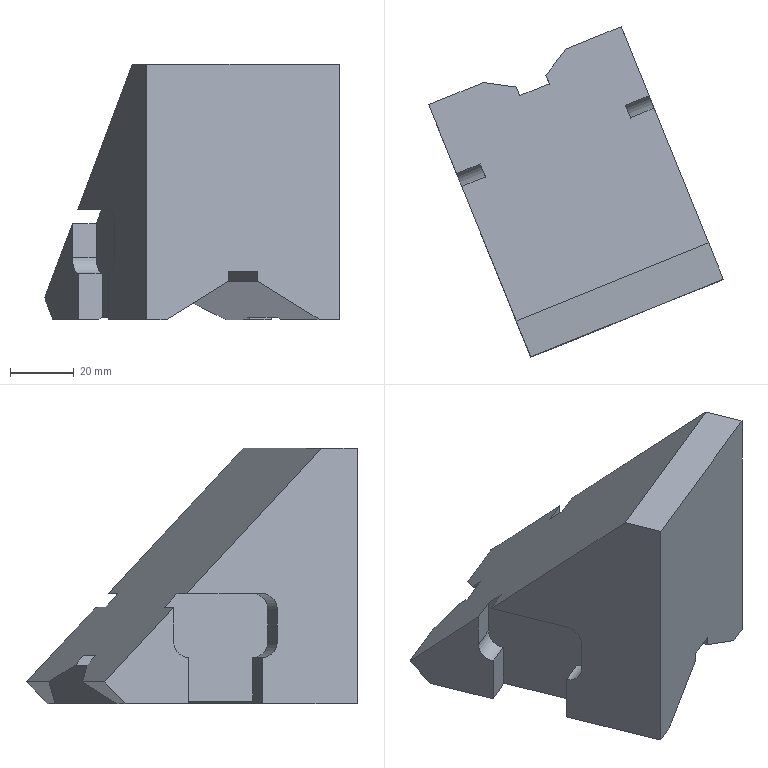Part | NX | features solid 2 | 1 solid | 36 faces | box 92.211 x 103.489 x 80 mm | volume 218804 mm3 | plane 30 | cylinder 6 | commonest cylinder face diameters 10 x6
STEP:
#1=CARTESIAN_POINT('',(-698.833,418.768,71.5));
#2=VERTEX_POINT('',#1);
#3=CARTESIAN_POINT('',(-689.172,394.857,71.5));
#4=VERTEX_POINT('',#3);
#5=CARTESIAN_POINT('',(-697.496,415.46,71.5));
#6=DIRECTION('',(0.3746,-0.9272,0.));
#7=VECTOR('',#6,1000.);
#8=LINE('',#5,#7);
#9=EDGE_CURVE('',#2,#4,#8,.T.);
#10=ORIENTED_EDGE('',*,*,#9,.T.);
#11=CARTESIAN_POINT('',(-696.589,391.86,71.5));
#12=VERTEX_POINT('',#11);
#13=CARTESIAN_POINT('',(-696.589,391.86,71.5));
#14=DIRECTION('',(0.9272,0.3746,0.));
#15=VECTOR('',#14,1000.);
#16=LINE('',#13,#15);
#17=EDGE_CURVE('',#12,#4,#16,.T.);
#18=ORIENTED_EDGE('',*,*,#17,.F.);
#19=CARTESIAN_POINT('',(-706.243,415.753,71.5));
#20=VERTEX_POINT('',#19);
#21=CARTESIAN_POINT('',(-704.914,412.464,71.5));
#22=DIRECTION('',(0.3746,-0.9272,0.));
#23=VECTOR('',#22,1000.);
#24=LINE('',#21,#23);
#25=EDGE_CURVE('',#20,#12,#24,.T.);
#26=ORIENTED_EDGE('',*,*,#25,.F.);
#27=CARTESIAN_POINT('',(-706.251,415.749,71.5));
#28=DIRECTION('',(-0.9262,-0.3769,0.));
#29=VECTOR('',#28,1000.);
#30=LINE('',#27,#29);
#31=EDGE_CURVE('',#2,#20,#30,.T.);
#32=ORIENTED_EDGE('',*,*,#31,.F.);
#33=EDGE_LOOP('',(#10,#18,#26,#32));
#34=FACE_BOUND('',#33,.T.);
#35=CARTESIAN_POINT('',(-704.914,412.464,71.5));
#36=DIRECTION('',(0.,0.,-1.));
#37=DIRECTION('',(0.3746,-0.9272,0.));
#38=AXIS2_PLACEMENT_3D('',#35,#36,#37);
#39=PLANE('',#38);
#40=ADVANCED_FACE('',(#34),#39,.T.);
#41=CARTESIAN_POINT('',(-700.41,422.673,67.289));
#42=VERTEX_POINT('',#41);
#43=CARTESIAN_POINT('',(-707.828,419.676,67.269));
#44=VERTEX_POINT('',#43);
#45=CARTESIAN_POINT('',(-707.839,419.671,67.269));
#46=DIRECTION('',(-0.9272,-0.3746,-0.002505));
#47=VECTOR('',#46,1000.);
#48=LINE('',#45,#47);
#49=EDGE_CURVE('',#42,#44,#48,.T.);
#50=ORIENTED_EDGE('',*,*,#49,.T.);
#51=CARTESIAN_POINT('',(-707.828,419.676,56.5));
#52=VERTEX_POINT('',#51);
#53=CARTESIAN_POINT('',(-707.828,419.676,62.23));
#54=DIRECTION('',(0.,0.,-1.));
#55=VECTOR('',#54,1000.);
#56=LINE('',#53,#55);
#57=EDGE_CURVE('',#44,#52,#56,.T.);
#58=ORIENTED_EDGE('',*,*,#57,.T.);
#59=CARTESIAN_POINT('',(-700.41,422.673,56.5));
#60=VERTEX_POINT('',#59);
#61=CARTESIAN_POINT('',(-707.828,419.676,56.5));
#62=DIRECTION('',(0.9272,0.3746,0.));
#63=VECTOR('',#62,1000.);
#64=LINE('',#61,#63);
#65=EDGE_CURVE('',#52,#60,#64,.T.);
#66=ORIENTED_EDGE('',*,*,#65,.T.);
#67=CARTESIAN_POINT('',(-700.41,422.673,62.23));
#68=DIRECTION('',(0.,0.,-1.));
#69=VECTOR('',#68,1000.);
#70=LINE('',#67,#69);
#71=EDGE_CURVE('',#42,#60,#70,.T.);
#72=ORIENTED_EDGE('',*,*,#71,.F.);
#73=EDGE_LOOP('',(#50,#58,#66,#72));
#74=FACE_BOUND('',#73,.T.);
#75=CARTESIAN_POINT('',(-707.828,419.676,62.23));
#76=DIRECTION('',(-0.3746,0.9272,0.));
#77=DIRECTION('',(0.,0.,-1.));
#78=AXIS2_PLACEMENT_3D('',#75,#76,#77);
#79=PLANE('',#78);
#80=ADVANCED_FACE('',(#74),#79,.F.);
#81=CARTESIAN_POINT('',(-753.26,401.32,67.146));
#82=VERTEX_POINT('',#81);
#83=CARTESIAN_POINT('',(-760.677,398.323,67.126));
#84=VERTEX_POINT('',#83);
#85=CARTESIAN_POINT('',(-760.689,398.319,67.126));
#86=DIRECTION('',(-0.9272,-0.3746,-0.002505));
#87=VECTOR('',#86,1000.);
#88=LINE('',#85,#87);
#89=EDGE_CURVE('',#82,#84,#88,.T.);
#90=ORIENTED_EDGE('',*,*,#89,.T.);
#91=CARTESIAN_POINT('',(-760.677,398.323,56.5));
#92=VERTEX_POINT('',#91);
#93=CARTESIAN_POINT('',(-760.677,398.323,62.23));
#94=DIRECTION('',(0.,0.,-1.));
#95=VECTOR('',#94,1000.);
#96=LINE('',#93,#95);
#97=EDGE_CURVE('',#84,#92,#96,.T.);
#98=ORIENTED_EDGE('',*,*,#97,.T.);
#99=CARTESIAN_POINT('',(-753.26,401.32,56.5));
#100=VERTEX_POINT('',#99);
#101=CARTESIAN_POINT('',(-760.677,398.323,56.5));
#102=DIRECTION('',(0.9272,0.3746,0.));
#103=VECTOR('',#102,1000.);
#104=LINE('',#101,#103);
#105=EDGE_CURVE('',#92,#100,#104,.T.);
#106=ORIENTED_EDGE('',*,*,#105,.T.);
#107=CARTESIAN_POINT('',(-753.26,401.32,62.23));
#108=DIRECTION('',(0.,0.,-1.));
#109=VECTOR('',#108,1000.);
#110=LINE('',#107,#109);
#111=EDGE_CURVE('',#82,#100,#110,.T.);
#112=ORIENTED_EDGE('',*,*,#111,.F.);
#113=EDGE_LOOP('',(#90,#98,#106,#112));
#114=FACE_BOUND('',#113,.T.);
#115=CARTESIAN_POINT('',(-760.677,398.323,62.23));
#116=DIRECTION('',(-0.3746,0.9272,0.));
#117=DIRECTION('',(0.,0.,-1.));
#118=AXIS2_PLACEMENT_3D('',#115,#116,#117);
#119=PLANE('',#118);
#120=ADVANCED_FACE('',(#114),#119,.F.);
#121=CARTESIAN_POINT('',(-751.629,397.283,71.5));
#122=VERTEX_POINT('',#121);
#123=CARTESIAN_POINT('',(-742.021,373.504,71.5));
#124=VERTEX_POINT('',#123);
#125=CARTESIAN_POINT('',(-750.346,394.108,71.5));
#126=DIRECTION('',(0.3746,-0.9272,0.));
#127=VECTOR('',#126,1000.);
#128=LINE('',#125,#127);
#129=EDGE_CURVE('',#122,#124,#128,.T.);
#130=ORIENTED_EDGE('',*,*,#129,.T.);
#131=CARTESIAN_POINT('',(-749.439,370.508,71.5));
#132=VERTEX_POINT('',#131);
#133=CARTESIAN_POINT('',(-749.439,370.508,71.5));
#134=DIRECTION('',(0.9272,0.3746,0.));
#135=VECTOR('',#134,1000.);
#136=LINE('',#133,#135);
#137=EDGE_CURVE('',#132,#124,#136,.T.);
#138=ORIENTED_EDGE('',*,*,#137,.F.);
#139=CARTESIAN_POINT('',(-759.039,394.268,71.5));
#140=VERTEX_POINT('',#139);
#141=CARTESIAN_POINT('',(-757.763,391.111,71.5));
#142=DIRECTION('',(0.3746,-0.9272,0.));
#143=VECTOR('',#142,1000.);
#144=LINE('',#141,#143);
#145=EDGE_CURVE('',#140,#132,#144,.T.);
#146=ORIENTED_EDGE('',*,*,#145,.F.);
#147=CARTESIAN_POINT('',(-759.046,394.264,71.5));
#148=DIRECTION('',(-0.9262,-0.3769,0.));
#149=VECTOR('',#148,1000.);
#150=LINE('',#147,#149);
#151=EDGE_CURVE('',#122,#140,#150,.T.);
#152=ORIENTED_EDGE('',*,*,#151,.F.);
#153=EDGE_LOOP('',(#130,#138,#146,#152));
#154=FACE_BOUND('',#153,.T.);
#155=CARTESIAN_POINT('',(-757.763,391.111,71.5));
#156=DIRECTION('',(0.,0.,-1.));
#157=DIRECTION('',(0.3746,-0.9272,0.));
#158=AXIS2_PLACEMENT_3D('',#155,#156,#157);
#159=PLANE('',#158);
#160=ADVANCED_FACE('',(#154),#159,.T.);
#161=CARTESIAN_POINT('',(-741.953,425.39,49.113));
#162=VERTEX_POINT('',#161);
#163=CARTESIAN_POINT('',(-711.954,351.139,49.113));
#164=VERTEX_POINT('',#163);
#165=CARTESIAN_POINT('',(-743.796,429.95,49.113));
#166=DIRECTION('',(0.3746,-0.9272,0.));
#167=VECTOR('',#166,1000.);
#168=LINE('',#165,#167);
#169=EDGE_CURVE('',#162,#164,#168,.T.);
#170=ORIENTED_EDGE('',*,*,#169,.T.);
#171=CARTESIAN_POINT('',(-731.406,343.28,37.));
#172=VERTEX_POINT('',#171);
#173=CARTESIAN_POINT('',(-711.954,351.139,49.113));
#174=DIRECTION('',(-0.803,-0.3244,-0.5));
#175=VECTOR('',#174,1000.);
#176=LINE('',#173,#175);
#177=EDGE_CURVE('',#164,#172,#176,.T.);
#178=ORIENTED_EDGE('',*,*,#177,.T.);
#179=CARTESIAN_POINT('',(-743.394,372.95,37.));
#180=VERTEX_POINT('',#179);
#181=CARTESIAN_POINT('',(-763.248,422.091,37.));
#182=DIRECTION('',(0.3746,-0.9272,0.));
#183=VECTOR('',#182,1000.);
#184=LINE('',#181,#183);
#185=EDGE_CURVE('',#180,#172,#184,.T.);
#186=ORIENTED_EDGE('',*,*,#185,.F.);
#187=CARTESIAN_POINT('',(-742.021,373.504,37.855));
#188=VERTEX_POINT('',#187);
#189=CARTESIAN_POINT('',(-723.941,380.809,49.113));
#190=DIRECTION('',(-0.803,-0.3244,-0.5));
#191=VECTOR('',#190,1000.);
#192=LINE('',#189,#191);
#193=EDGE_CURVE('',#188,#180,#192,.T.);
#194=ORIENTED_EDGE('',*,*,#193,.F.);
#195=CARTESIAN_POINT('',(-751.387,396.684,37.855));
#196=VERTEX_POINT('',#195);
#197=CARTESIAN_POINT('',(-761.876,422.645,37.855));
#198=DIRECTION('',(-0.3746,0.9272,0.));
#199=VECTOR('',#198,1000.);
#200=LINE('',#197,#199);
#201=EDGE_CURVE('',#188,#196,#200,.T.);
#202=ORIENTED_EDGE('',*,*,#201,.T.);
#203=CARTESIAN_POINT('',(-752.759,396.13,37.));
#204=VERTEX_POINT('',#203);
#205=CARTESIAN_POINT('',(-733.307,403.989,49.113));
#206=DIRECTION('',(0.803,0.3244,0.5));
#207=VECTOR('',#206,1000.);
#208=LINE('',#205,#207);
#209=EDGE_CURVE('',#204,#196,#208,.T.);
#210=ORIENTED_EDGE('',*,*,#209,.F.);
#211=CARTESIAN_POINT('',(-760.783,415.991,37.));
#212=VERTEX_POINT('',#211);
#213=CARTESIAN_POINT('',(-763.248,422.091,37.));
#214=DIRECTION('',(0.3746,-0.9272,0.));
#215=VECTOR('',#214,1000.);
#216=LINE('',#213,#215);
#217=EDGE_CURVE('',#212,#204,#216,.T.);
#218=ORIENTED_EDGE('',*,*,#217,.F.);
#219=CARTESIAN_POINT('',(-752.317,426.827,43.876));
#220=VERTEX_POINT('',#219);
#221=CARTESIAN_POINT('',(-747.231,433.337,48.006));
#222=DIRECTION('',(0.5507,0.7048,0.4472));
#223=VECTOR('',#222,1000.);
#224=LINE('',#221,#223);
#225=EDGE_CURVE('',#212,#220,#224,.T.);
#226=ORIENTED_EDGE('',*,*,#225,.T.);
#227=CARTESIAN_POINT('',(-743.895,425.659,48.132));
#228=DIRECTION('',(-0.8858,0.1228,-0.4476));
#229=VECTOR('',#228,1000.);
#230=LINE('',#227,#229);
#231=EDGE_CURVE('',#162,#220,#230,.T.);
#232=ORIENTED_EDGE('',*,*,#231,.F.);
#233=EDGE_LOOP('',(#170,#178,#186,#194,#202,#210,#218,#226,#232));
#234=FACE_BOUND('',#233,.T.);
#235=CARTESIAN_POINT('',(-743.796,429.95,49.113));
#236=DIRECTION('',(0.4636,0.1873,-0.866));
#237=DIRECTION('',(-0.6969,-0.5265,-0.4869));
#238=AXIS2_PLACEMENT_3D('',#235,#236,#237);
#239=PLANE('',#238);
#240=ADVANCED_FACE('',(#234),#239,.T.);
#241=CARTESIAN_POINT('',(-769.396,419.902,43.852));
#242=VERTEX_POINT('',#241);
#243=CARTESIAN_POINT('',(-766.829,413.548,37.));
#244=VERTEX_POINT('',#243);
#245=CARTESIAN_POINT('',(-767.796,415.943,39.582));
#246=DIRECTION('',(0.2649,-0.6556,-0.7071));
#247=VECTOR('',#246,1000.);
#248=LINE('',#245,#247);
#249=EDGE_CURVE('',#242,#244,#248,.T.);
#250=ORIENTED_EDGE('',*,*,#249,.T.);
#251=CARTESIAN_POINT('',(-758.804,393.687,37.));
#252=VERTEX_POINT('',#251);
#253=CARTESIAN_POINT('',(-769.293,419.648,37.));
#254=DIRECTION('',(0.3746,-0.9272,0.));
#255=VECTOR('',#254,1000.);
#256=LINE('',#253,#255);
#257=EDGE_CURVE('',#244,#252,#256,.T.);
#258=ORIENTED_EDGE('',*,*,#257,.T.);
#259=CARTESIAN_POINT('',(-758.804,393.687,51.5));
#260=VERTEX_POINT('',#259);
#261=CARTESIAN_POINT('',(-758.804,393.687,37.));
#262=DIRECTION('',(0.,0.,1.));
#263=VECTOR('',#262,1000.);
#264=LINE('',#261,#263);
#265=EDGE_CURVE('',#252,#260,#264,.T.);
#266=ORIENTED_EDGE('',*,*,#265,.T.);
#267=CARTESIAN_POINT('',(-758.804,393.687,56.5));
#268=DIRECTION('',(-0.9272,-0.3746,0.));
#269=DIRECTION('',(0.3069,-0.7595,0.5736));
#270=AXIS2_PLACEMENT_3D('',#267,#268,#269);
#271=CIRCLE('',#270,5.);
#272=EDGE_CURVE('',#92,#260,#271,.T.);
#273=ORIENTED_EDGE('',*,*,#272,.F.);
#274=ORIENTED_EDGE('',*,*,#97,.F.);
#275=CARTESIAN_POINT('',(-770.628,422.952,40.563));
#276=DIRECTION('',(0.2649,-0.6556,0.7071));
#277=VECTOR('',#276,1000.);
#278=LINE('',#275,#277);
#279=EDGE_CURVE('',#242,#84,#278,.T.);
#280=ORIENTED_EDGE('',*,*,#279,.F.);
#281=EDGE_LOOP('',(#250,#258,#266,#273,#274,#280));
#282=FACE_BOUND('',#281,.T.);
#283=CARTESIAN_POINT('',(-769.293,419.648,37.));
#284=DIRECTION('',(-0.9272,-0.3746,0.));
#285=DIRECTION('',(-0.1583,0.3918,0.9063));
#286=AXIS2_PLACEMENT_3D('',#283,#284,#285);
#287=PLANE('',#286);
#288=ADVANCED_FACE('',(#282),#287,.T.);
#289=ORIENTED_EDGE('',*,*,#145,.T.);
#290=CARTESIAN_POINT('',(-747.566,365.872,66.5));
#291=VERTEX_POINT('',#290);
#292=CARTESIAN_POINT('',(-749.439,370.508,66.5));
#293=DIRECTION('',(-0.9272,-0.3746,0.));
#294=DIRECTION('',(0.3069,-0.7595,0.5736));
#295=AXIS2_PLACEMENT_3D('',#292,#293,#294);
#296=CIRCLE('',#295,5.);
#297=EDGE_CURVE('',#291,#132,#296,.T.);
#298=ORIENTED_EDGE('',*,*,#297,.F.);
#299=CARTESIAN_POINT('',(-747.566,365.872,56.5));
#300=VERTEX_POINT('',#299);
#301=CARTESIAN_POINT('',(-747.566,365.872,66.5));
#302=DIRECTION('',(0.,0.,-1.));
#303=VECTOR('',#302,1000.);
#304=LINE('',#301,#303);
#305=EDGE_CURVE('',#291,#300,#304,.T.);
#306=ORIENTED_EDGE('',*,*,#305,.T.);
#307=CARTESIAN_POINT('',(-749.439,370.508,51.5));
#308=VERTEX_POINT('',#307);
#309=CARTESIAN_POINT('',(-749.439,370.508,56.5));
#310=DIRECTION('',(-0.9272,-0.3746,0.));
#311=DIRECTION('',(0.3069,-0.7595,0.5736));
#312=AXIS2_PLACEMENT_3D('',#309,#310,#311);
#313=CIRCLE('',#312,5.);
#314=EDGE_CURVE('',#308,#300,#313,.T.);
#315=ORIENTED_EDGE('',*,*,#314,.F.);
#316=CARTESIAN_POINT('',(-749.439,370.508,37.));
#317=VERTEX_POINT('',#316);
#318=CARTESIAN_POINT('',(-749.439,370.508,51.5));
#319=DIRECTION('',(0.,0.,-1.));
#320=VECTOR('',#319,1000.);
#321=LINE('',#318,#320);
#322=EDGE_CURVE('',#308,#317,#321,.T.);
#323=ORIENTED_EDGE('',*,*,#322,.T.);
#324=CARTESIAN_POINT('',(-737.452,340.838,37.));
#325=VERTEX_POINT('',#324);
#326=CARTESIAN_POINT('',(-769.293,419.648,37.));
#327=DIRECTION('',(0.3746,-0.9272,0.));
#328=VECTOR('',#327,1000.);
#329=LINE('',#326,#328);
#330=EDGE_CURVE('',#317,#325,#329,.T.);
#331=ORIENTED_EDGE('',*,*,#330,.T.);
#332=CARTESIAN_POINT('',(-737.452,340.838,117.));
#333=VERTEX_POINT('',#332);
#334=CARTESIAN_POINT('',(-737.452,340.838,37.));
#335=DIRECTION('',(0.,0.,1.));
#336=VECTOR('',#335,1000.);
#337=LINE('',#334,#336);
#338=EDGE_CURVE('',#325,#333,#337,.T.);
#339=ORIENTED_EDGE('',*,*,#338,.T.);
#340=CARTESIAN_POINT('',(-741.994,352.081,117.));
#341=VERTEX_POINT('',#340);
#342=CARTESIAN_POINT('',(-769.293,419.648,117.));
#343=DIRECTION('',(0.3746,-0.9272,0.));
#344=VECTOR('',#343,1000.);
#345=LINE('',#342,#344);
#346=EDGE_CURVE('',#341,#333,#345,.T.);
#347=ORIENTED_EDGE('',*,*,#346,.F.);
#348=CARTESIAN_POINT('',(-770.628,422.952,40.563));
#349=DIRECTION('',(0.2649,-0.6556,0.7071));
#350=VECTOR('',#349,1000.);
#351=LINE('',#348,#350);
#352=EDGE_CURVE('',#140,#341,#351,.T.);
#353=ORIENTED_EDGE('',*,*,#352,.F.);
#354=EDGE_LOOP('',(#289,#298,#306,#315,#323,#331,#339,#347,#353));
#355=FACE_BOUND('',#354,.T.);
#356=CARTESIAN_POINT('',(-769.293,419.648,37.));
#357=DIRECTION('',(-0.9272,-0.3746,0.));
#358=DIRECTION('',(-0.1583,0.3918,0.9063));
#359=AXIS2_PLACEMENT_3D('',#356,#357,#358);
#360=PLANE('',#359);
#361=ADVANCED_FACE('',(#355),#360,.T.);
#362=CARTESIAN_POINT('',(-726.294,437.379,43.911));
#363=VERTEX_POINT('',#362);
#364=CARTESIAN_POINT('',(-712.607,435.455,37.));
#365=VERTEX_POINT('',#364);
#366=CARTESIAN_POINT('',(-715.213,435.822,38.316));
#367=DIRECTION('',(0.8857,-0.1245,-0.4472));
#368=VECTOR('',#367,1000.);
#369=LINE('',#366,#368);
#370=EDGE_CURVE('',#363,#365,#369,.T.);
#371=ORIENTED_EDGE('',*,*,#370,.T.);
#372=CARTESIAN_POINT('',(-704.582,415.594,37.));
#373=VERTEX_POINT('',#372);
#374=CARTESIAN_POINT('',(-715.071,441.555,37.));
#375=DIRECTION('',(0.3746,-0.9272,0.));
#376=VECTOR('',#375,1000.);
#377=LINE('',#374,#376);
#378=EDGE_CURVE('',#365,#373,#377,.T.);
#379=ORIENTED_EDGE('',*,*,#378,.T.);
#380=CARTESIAN_POINT('',(-705.955,415.04,37.855));
#381=VERTEX_POINT('',#380);
#382=CARTESIAN_POINT('',(-704.582,415.594,37.));
#383=DIRECTION('',(0.803,0.3244,-0.5));
#384=VECTOR('',#383,1000.);
#385=LINE('',#382,#384);
#386=EDGE_CURVE('',#381,#373,#385,.T.);
#387=ORIENTED_EDGE('',*,*,#386,.F.);
#388=CARTESIAN_POINT('',(-696.589,391.86,37.855));
#389=VERTEX_POINT('',#388);
#390=CARTESIAN_POINT('',(-716.444,441.001,37.855));
#391=DIRECTION('',(-0.3746,0.9272,0.));
#392=VECTOR('',#391,1000.);
#393=LINE('',#390,#392);
#394=EDGE_CURVE('',#389,#381,#393,.T.);
#395=ORIENTED_EDGE('',*,*,#394,.F.);
#396=CARTESIAN_POINT('',(-695.217,392.415,37.));
#397=VERTEX_POINT('',#396);
#398=CARTESIAN_POINT('',(-695.217,392.415,37.));
#399=DIRECTION('',(-0.803,-0.3244,0.5));
#400=VECTOR('',#399,1000.);
#401=LINE('',#398,#400);
#402=EDGE_CURVE('',#397,#389,#401,.T.);
#403=ORIENTED_EDGE('',*,*,#402,.F.);
#404=CARTESIAN_POINT('',(-683.23,362.745,37.));
#405=VERTEX_POINT('',#404);
#406=CARTESIAN_POINT('',(-715.071,441.555,37.));
#407=DIRECTION('',(0.3746,-0.9272,0.));
#408=VECTOR('',#407,1000.);
#409=LINE('',#406,#408);
#410=EDGE_CURVE('',#397,#405,#409,.T.);
#411=ORIENTED_EDGE('',*,*,#410,.T.);
#412=CARTESIAN_POINT('',(-702.682,354.885,49.113));
#413=VERTEX_POINT('',#412);
#414=CARTESIAN_POINT('',(-683.23,362.745,37.));
#415=DIRECTION('',(-0.803,-0.3244,0.5));
#416=VECTOR('',#415,1000.);
#417=LINE('',#414,#416);
#418=EDGE_CURVE('',#405,#413,#417,.T.);
#419=ORIENTED_EDGE('',*,*,#418,.T.);
#420=CARTESIAN_POINT('',(-732.691,429.159,49.113));
#421=VERTEX_POINT('',#420);
#422=CARTESIAN_POINT('',(-734.524,433.696,49.113));
#423=DIRECTION('',(0.3746,-0.9272,0.));
#424=VECTOR('',#423,1000.);
#425=LINE('',#422,#424);
#426=EDGE_CURVE('',#421,#413,#425,.T.);
#427=ORIENTED_EDGE('',*,*,#426,.F.);
#428=CARTESIAN_POINT('',(-719.589,445.994,38.458));
#429=DIRECTION('',(-0.5495,-0.706,0.4468));
#430=VECTOR('',#429,1000.);
#431=LINE('',#428,#430);
#432=EDGE_CURVE('',#363,#421,#431,.T.);
#433=ORIENTED_EDGE('',*,*,#432,.F.);
#434=EDGE_LOOP('',(#371,#379,#387,#395,#403,#411,#419,#427,#433));
#435=FACE_BOUND('',#434,.T.);
#436=CARTESIAN_POINT('',(-715.071,441.555,37.));
#437=DIRECTION('',(-0.4636,-0.1873,-0.866));
#438=DIRECTION('',(-0.8671,-0.1054,0.4869));
#439=AXIS2_PLACEMENT_3D('',#436,#437,#438);
#440=PLANE('',#439);
#441=ADVANCED_FACE('',(#435),#440,.T.);
#442=CARTESIAN_POINT('',(-709.159,444.327,43.934));
#443=VERTEX_POINT('',#442);
#444=CARTESIAN_POINT('',(-710.391,447.377,40.644));
#445=DIRECTION('',(0.2649,-0.6556,0.7071));
#446=VECTOR('',#445,1000.);
#447=LINE('',#444,#446);
#448=EDGE_CURVE('',#443,#42,#447,.T.);
#449=ORIENTED_EDGE('',*,*,#448,.T.);
#450=ORIENTED_EDGE('',*,*,#71,.T.);
#451=CARTESIAN_POINT('',(-698.537,418.037,51.5));
#452=VERTEX_POINT('',#451);
#453=CARTESIAN_POINT('',(-698.537,418.037,56.5));
#454=DIRECTION('',(-0.9272,-0.3746,0.));
#455=DIRECTION('',(0.3069,-0.7595,0.5736));
#456=AXIS2_PLACEMENT_3D('',#453,#454,#455);
#457=CIRCLE('',#456,5.);
#458=EDGE_CURVE('',#60,#452,#457,.T.);
#459=ORIENTED_EDGE('',*,*,#458,.T.);
#460=CARTESIAN_POINT('',(-698.537,418.037,37.));
#461=VERTEX_POINT('',#460);
#462=CARTESIAN_POINT('',(-698.537,418.037,37.));
#463=DIRECTION('',(0.,0.,1.));
#464=VECTOR('',#463,1000.);
#465=LINE('',#462,#464);
#466=EDGE_CURVE('',#461,#452,#465,.T.);
#467=ORIENTED_EDGE('',*,*,#466,.F.);
#468=CARTESIAN_POINT('',(-706.562,437.898,37.));
#469=VERTEX_POINT('',#468);
#470=CARTESIAN_POINT('',(-709.026,443.998,37.));
#471=DIRECTION('',(0.3746,-0.9272,0.));
#472=VECTOR('',#471,1000.);
#473=LINE('',#470,#472);
#474=EDGE_CURVE('',#469,#461,#473,.T.);
#475=ORIENTED_EDGE('',*,*,#474,.F.);
#476=CARTESIAN_POINT('',(-707.529,440.292,39.582));
#477=DIRECTION('',(0.2649,-0.6556,-0.7071));
#478=VECTOR('',#477,1000.);
#479=LINE('',#476,#478);
#480=EDGE_CURVE('',#443,#469,#479,.T.);
#481=ORIENTED_EDGE('',*,*,#480,.F.);
#482=EDGE_LOOP('',(#449,#450,#459,#467,#475,#481));
#483=FACE_BOUND('',#482,.T.);
#484=CARTESIAN_POINT('',(-709.026,443.998,37.));
#485=DIRECTION('',(-0.9272,-0.3746,0.));
#486=DIRECTION('',(-0.3395,0.8403,-0.4226));
#487=AXIS2_PLACEMENT_3D('',#484,#485,#486);
#488=PLANE('',#487);
#489=ADVANCED_FACE('',(#483),#488,.F.);
#490=CARTESIAN_POINT('',(-681.788,376.581,117.));
#491=VERTEX_POINT('',#490);
#492=CARTESIAN_POINT('',(-710.391,447.377,40.644));
#493=DIRECTION('',(0.2649,-0.6556,0.7071));
#494=VECTOR('',#493,1000.);
#495=LINE('',#492,#494);
#496=EDGE_CURVE('',#2,#491,#495,.T.);
#497=ORIENTED_EDGE('',*,*,#496,.T.);
#498=CARTESIAN_POINT('',(-677.185,365.187,117.));
#499=VERTEX_POINT('',#498);
#500=CARTESIAN_POINT('',(-709.026,443.998,117.));
#501=DIRECTION('',(0.3746,-0.9272,0.));
#502=VECTOR('',#501,1000.);
#503=LINE('',#500,#502);
#504=EDGE_CURVE('',#491,#499,#503,.T.);
#505=ORIENTED_EDGE('',*,*,#504,.T.);
#506=CARTESIAN_POINT('',(-677.185,365.187,37.));
#507=VERTEX_POINT('',#506);
#508=CARTESIAN_POINT('',(-677.185,365.187,37.));
#509=DIRECTION('',(0.,0.,1.));
#510=VECTOR('',#509,1000.);
#511=LINE('',#508,#510);
#512=EDGE_CURVE('',#507,#499,#511,.T.);
#513=ORIENTED_EDGE('',*,*,#512,.F.);
#514=CARTESIAN_POINT('',(-689.172,394.857,37.));
#515=VERTEX_POINT('',#514);
#516=CARTESIAN_POINT('',(-709.026,443.998,37.));
#517=DIRECTION('',(0.3746,-0.9272,0.));
#518=VECTOR('',#517,1000.);
#519=LINE('',#516,#518);
#520=EDGE_CURVE('',#515,#507,#519,.T.);
#521=ORIENTED_EDGE('',*,*,#520,.F.);
#522=CARTESIAN_POINT('',(-689.172,394.857,51.5));
#523=VERTEX_POINT('',#522);
#524=CARTESIAN_POINT('',(-689.172,394.857,51.5));
#525=DIRECTION('',(0.,0.,-1.));
#526=VECTOR('',#525,1000.);
#527=LINE('',#524,#526);
#528=EDGE_CURVE('',#523,#515,#527,.T.);
#529=ORIENTED_EDGE('',*,*,#528,.F.);
#530=CARTESIAN_POINT('',(-687.299,390.221,56.5));
#531=VERTEX_POINT('',#530);
#532=CARTESIAN_POINT('',(-689.172,394.857,56.5));
#533=DIRECTION('',(-0.9272,-0.3746,0.));
#534=DIRECTION('',(0.3069,-0.7595,0.5736));
#535=AXIS2_PLACEMENT_3D('',#532,#533,#534);
#536=CIRCLE('',#535,5.);
#537=EDGE_CURVE('',#523,#531,#536,.T.);
#538=ORIENTED_EDGE('',*,*,#537,.T.);
#539=CARTESIAN_POINT('',(-687.299,390.221,66.5));
#540=VERTEX_POINT('',#539);
#541=CARTESIAN_POINT('',(-687.299,390.221,66.5));
#542=DIRECTION('',(0.,0.,-1.));
#543=VECTOR('',#542,1000.);
#544=LINE('',#541,#543);
#545=EDGE_CURVE('',#540,#531,#544,.T.);
#546=ORIENTED_EDGE('',*,*,#545,.F.);
#547=CARTESIAN_POINT('',(-689.172,394.857,66.5));
#548=DIRECTION('',(-0.9272,-0.3746,0.));
#549=DIRECTION('',(0.3069,-0.7595,0.5736));
#550=AXIS2_PLACEMENT_3D('',#547,#548,#549);
#551=CIRCLE('',#550,5.);
#552=EDGE_CURVE('',#540,#4,#551,.T.);
#553=ORIENTED_EDGE('',*,*,#552,.T.);
#554=ORIENTED_EDGE('',*,*,#9,.F.);
#555=EDGE_LOOP('',(#497,#505,#513,#521,#529,#538,#546,#553,#554));
#556=FACE_BOUND('',#555,.T.);
#557=CARTESIAN_POINT('',(-709.026,443.998,37.));
#558=DIRECTION('',(-0.9272,-0.3746,0.));
#559=DIRECTION('',(-0.3395,0.8403,-0.4226));
#560=AXIS2_PLACEMENT_3D('',#557,#558,#559);
#561=PLANE('',#560);
#562=ADVANCED_FACE('',(#556),#561,.F.);
#563=CARTESIAN_POINT('',(-731.609,426.483,52.));
#564=VERTEX_POINT('',#563);
#565=CARTESIAN_POINT('',(-733.066,430.089,48.11));
#566=DIRECTION('',(-0.2649,0.6556,-0.7071));
#567=VECTOR('',#566,1000.);
#568=LINE('',#565,#567);
#569=EDGE_CURVE('',#564,#421,#568,.T.);
#570=ORIENTED_EDGE('',*,*,#569,.T.);
#571=ORIENTED_EDGE('',*,*,#426,.T.);
#572=CARTESIAN_POINT('',(-702.682,354.885,52.));
#573=VERTEX_POINT('',#572);
#574=CARTESIAN_POINT('',(-702.682,354.885,52.));
#575=DIRECTION('',(0.,0.,-1.));
#576=VECTOR('',#575,1000.);
#577=LINE('',#574,#576);
#578=EDGE_CURVE('',#573,#413,#577,.T.);
#579=ORIENTED_EDGE('',*,*,#578,.F.);
#580=CARTESIAN_POINT('',(-734.524,433.696,52.));
#581=DIRECTION('',(0.3746,-0.9272,0.));
#582=VECTOR('',#581,1000.);
#583=LINE('',#580,#582);
#584=EDGE_CURVE('',#564,#573,#583,.T.);
#585=ORIENTED_EDGE('',*,*,#584,.F.);
#586=EDGE_LOOP('',(#570,#571,#579,#585));
#587=FACE_BOUND('',#586,.T.);
#588=CARTESIAN_POINT('',(-734.524,433.696,52.));
#589=DIRECTION('',(0.9272,0.3746,0.));
#590=DIRECTION('',(0.1583,-0.3918,-0.9063));
#591=AXIS2_PLACEMENT_3D('',#588,#589,#590);
#592=PLANE('',#591);
#593=ADVANCED_FACE('',(#587),#592,.F.);
#594=ORIENTED_EDGE('',*,*,#584,.T.);
#595=CARTESIAN_POINT('',(-711.954,351.139,52.));
#596=VERTEX_POINT('',#595);
#597=CARTESIAN_POINT('',(-702.682,354.885,52.));
#598=DIRECTION('',(-0.9272,-0.3746,0.));
#599=VECTOR('',#598,1000.);
#600=LINE('',#597,#599);
#601=EDGE_CURVE('',#573,#596,#600,.T.);
#602=ORIENTED_EDGE('',*,*,#601,.T.);
#603=CARTESIAN_POINT('',(-740.872,422.713,52.));
#604=VERTEX_POINT('',#603);
#605=CARTESIAN_POINT('',(-743.796,429.95,52.));
#606=DIRECTION('',(0.3746,-0.9272,0.));
#607=VECTOR('',#606,1000.);
#608=LINE('',#605,#607);
#609=EDGE_CURVE('',#604,#596,#608,.T.);
#610=ORIENTED_EDGE('',*,*,#609,.F.);
#611=CARTESIAN_POINT('',(-731.591,426.49,52.));
#612=DIRECTION('',(-0.9262,-0.3769,0.));
#613=VECTOR('',#612,1000.);
#614=LINE('',#611,#613);
#615=EDGE_CURVE('',#564,#604,#614,.T.);
#616=ORIENTED_EDGE('',*,*,#615,.F.);
#617=EDGE_LOOP('',(#594,#602,#610,#616));
#618=FACE_BOUND('',#617,.T.);
#619=CARTESIAN_POINT('',(-734.524,433.696,52.));
#620=DIRECTION('',(0.,0.,-1.));
#621=DIRECTION('',(0.3746,-0.9272,0.));
#622=AXIS2_PLACEMENT_3D('',#619,#620,#621);
#623=PLANE('',#622);
#624=ADVANCED_FACE('',(#618),#623,.T.);
#625=CARTESIAN_POINT('',(-742.874,427.67,46.654));
#626=DIRECTION('',(0.2649,-0.6556,0.7071));
#627=VECTOR('',#626,1000.);
#628=LINE('',#625,#627);
#629=EDGE_CURVE('',#162,#604,#628,.T.);
#630=ORIENTED_EDGE('',*,*,#629,.T.);
#631=ORIENTED_EDGE('',*,*,#609,.T.);
#632=CARTESIAN_POINT('',(-711.954,351.139,49.113));
#633=DIRECTION('',(0.,0.,1.));
#634=VECTOR('',#633,1000.);
#635=LINE('',#632,#634);
#636=EDGE_CURVE('',#164,#596,#635,.T.);
#637=ORIENTED_EDGE('',*,*,#636,.F.);
#638=ORIENTED_EDGE('',*,*,#169,.F.);
#639=EDGE_LOOP('',(#630,#631,#637,#638));
#640=FACE_BOUND('',#639,.T.);
#641=CARTESIAN_POINT('',(-743.796,429.95,49.113));
#642=DIRECTION('',(-0.9272,-0.3746,0.));
#643=DIRECTION('',(-0.3395,0.8403,-0.4226));
#644=AXIS2_PLACEMENT_3D('',#641,#642,#643);
#645=PLANE('',#644);
#646=ADVANCED_FACE('',(#640),#645,.F.);
#647=CARTESIAN_POINT('',(-681.619,376.65,117.));
#648=DIRECTION('',(-0.9262,-0.3769,0.));
#649=VECTOR('',#648,1000.);
#650=LINE('',#647,#649);
#651=EDGE_CURVE('',#491,#341,#650,.T.);
#652=ORIENTED_EDGE('',*,*,#651,.T.);
#653=ORIENTED_EDGE('',*,*,#346,.T.);
#654=CARTESIAN_POINT('',(-737.452,340.838,117.));
#655=DIRECTION('',(-0.9272,-0.3746,0.));
#656=VECTOR('',#655,1000.);
#657=LINE('',#654,#656);
#658=EDGE_CURVE('',#499,#333,#657,.T.);
#659=ORIENTED_EDGE('',*,*,#658,.F.);
#660=ORIENTED_EDGE('',*,*,#504,.F.);
#661=EDGE_LOOP('',(#652,#653,#659,#660));
#662=FACE_BOUND('',#661,.T.);
#663=CARTESIAN_POINT('',(-709.026,443.998,117.));
#664=DIRECTION('',(0.,0.,-1.));
#665=DIRECTION('',(0.3746,-0.9272,0.));
#666=AXIS2_PLACEMENT_3D('',#663,#664,#665);
#667=PLANE('',#666);
#668=ADVANCED_FACE('',(#662),#667,.F.);
#669=CARTESIAN_POINT('',(-709.169,444.323,43.934));
#670=DIRECTION('',(0.9267,0.3758,0.001252));
#671=VECTOR('',#670,1000.);
#672=LINE('',#669,#671);
#673=EDGE_CURVE('',#363,#443,#672,.T.);
#674=ORIENTED_EDGE('',*,*,#673,.T.);
#675=ORIENTED_EDGE('',*,*,#480,.T.);
#676=CARTESIAN_POINT('',(-706.562,437.898,37.));
#677=DIRECTION('',(-0.9272,-0.3746,0.));
#678=VECTOR('',#677,1000.);
#679=LINE('',#676,#678);
#680=EDGE_CURVE('',#469,#365,#679,.T.);
#681=ORIENTED_EDGE('',*,*,#680,.T.);
#682=ORIENTED_EDGE('',*,*,#370,.F.);
#683=EDGE_LOOP('',(#674,#675,#681,#682));
#684=FACE_BOUND('',#683,.T.);
#685=CARTESIAN_POINT('',(-707.529,440.292,39.582));
#686=DIRECTION('',(0.2649,-0.6556,0.7071));
#687=DIRECTION('',(-0.2649,0.6556,0.7071));
#688=AXIS2_PLACEMENT_3D('',#685,#686,#687);
#689=PLANE('',#688);
#690=ADVANCED_FACE('',(#684),#689,.F.);
#691=CARTESIAN_POINT('',(-709.169,444.323,43.934));
#692=DIRECTION('',(0.9267,0.3758,0.001252));
#693=VECTOR('',#692,1000.);
#694=LINE('',#691,#693);
#695=EDGE_CURVE('',#242,#220,#694,.T.);
#696=ORIENTED_EDGE('',*,*,#695,.T.);
#697=ORIENTED_EDGE('',*,*,#225,.F.);
#698=CARTESIAN_POINT('',(-706.562,437.898,37.));
#699=DIRECTION('',(-0.9272,-0.3746,0.));
#700=VECTOR('',#699,1000.);
#701=LINE('',#698,#700);
#702=EDGE_CURVE('',#212,#244,#701,.T.);
#703=ORIENTED_EDGE('',*,*,#702,.T.);
#704=ORIENTED_EDGE('',*,*,#249,.F.);
#705=EDGE_LOOP('',(#696,#697,#703,#704));
#706=FACE_BOUND('',#705,.T.);
#707=CARTESIAN_POINT('',(-707.529,440.292,39.582));
#708=DIRECTION('',(0.2649,-0.6556,0.7071));
#709=DIRECTION('',(-0.2649,0.6556,0.7071));
#710=AXIS2_PLACEMENT_3D('',#707,#708,#709);
#711=PLANE('',#710);
#712=ADVANCED_FACE('',(#706),#711,.F.);
#713=ORIENTED_EDGE('',*,*,#25,.T.);
#714=CARTESIAN_POINT('',(-694.716,387.224,66.5));
#715=VERTEX_POINT('',#714);
#716=CARTESIAN_POINT('',(-696.589,391.86,66.5));
#717=DIRECTION('',(-0.9272,-0.3746,0.));
#718=DIRECTION('',(0.3069,-0.7595,0.5736));
#719=AXIS2_PLACEMENT_3D('',#716,#717,#718);
#720=CIRCLE('',#719,5.);
#721=EDGE_CURVE('',#715,#12,#720,.T.);
#722=ORIENTED_EDGE('',*,*,#721,.F.);
#723=CARTESIAN_POINT('',(-694.716,387.224,56.5));
#724=VERTEX_POINT('',#723);
#725=CARTESIAN_POINT('',(-694.716,387.224,66.5));
#726=DIRECTION('',(0.,0.,-1.));
#727=VECTOR('',#726,1000.);
#728=LINE('',#725,#727);
#729=EDGE_CURVE('',#715,#724,#728,.T.);
#730=ORIENTED_EDGE('',*,*,#729,.T.);
#731=CARTESIAN_POINT('',(-696.589,391.86,51.5));
#732=VERTEX_POINT('',#731);
#733=CARTESIAN_POINT('',(-696.589,391.86,56.5));
#734=DIRECTION('',(-0.9272,-0.3746,0.));
#735=DIRECTION('',(0.3069,-0.7595,0.5736));
#736=AXIS2_PLACEMENT_3D('',#733,#734,#735);
#737=CIRCLE('',#736,5.);
#738=EDGE_CURVE('',#732,#724,#737,.T.);
#739=ORIENTED_EDGE('',*,*,#738,.F.);
#740=CARTESIAN_POINT('',(-696.589,391.86,51.5));
#741=DIRECTION('',(0.,0.,-1.));
#742=VECTOR('',#741,1000.);
#743=LINE('',#740,#742);
#744=EDGE_CURVE('',#732,#389,#743,.T.);
#745=ORIENTED_EDGE('',*,*,#744,.T.);
#746=ORIENTED_EDGE('',*,*,#394,.T.);
#747=CARTESIAN_POINT('',(-705.955,415.04,51.5));
#748=VERTEX_POINT('',#747);
#749=CARTESIAN_POINT('',(-705.955,415.04,37.));
#750=DIRECTION('',(0.,0.,1.));
#751=VECTOR('',#750,1000.);
#752=LINE('',#749,#751);
#753=EDGE_CURVE('',#381,#748,#752,.T.);
#754=ORIENTED_EDGE('',*,*,#753,.T.);
#755=CARTESIAN_POINT('',(-705.955,415.04,56.5));
#756=DIRECTION('',(-0.9272,-0.3746,0.));
#757=DIRECTION('',(0.3069,-0.7595,0.5736));
#758=AXIS2_PLACEMENT_3D('',#755,#756,#757);
#759=CIRCLE('',#758,5.);
#760=EDGE_CURVE('',#52,#748,#759,.T.);
#761=ORIENTED_EDGE('',*,*,#760,.F.);
#762=ORIENTED_EDGE('',*,*,#57,.F.);
#763=CARTESIAN_POINT('',(-708.908,422.35,64.384));
#764=DIRECTION('',(-0.2649,0.6556,-0.7071));
#765=VECTOR('',#764,1000.);
#766=LINE('',#763,#765);
#767=EDGE_CURVE('',#20,#44,#766,.T.);
#768=ORIENTED_EDGE('',*,*,#767,.F.);
#769=EDGE_LOOP('',(#713,#722,#730,#739,#745,#746,#754,#761,#762,#768));
#770=FACE_BOUND('',#769,.T.);
#771=CARTESIAN_POINT('',(-705.955,415.04,56.5));
#772=DIRECTION('',(0.9272,0.3746,0.));
#773=DIRECTION('',(0.3395,-0.8403,0.4226));
#774=AXIS2_PLACEMENT_3D('',#771,#772,#773);
#775=PLANE('',#774);
#776=ADVANCED_FACE('',(#770),#775,.T.);
#777=CARTESIAN_POINT('',(-754.317,403.937,64.323));
#778=DIRECTION('',(-0.2649,0.6556,-0.7071));
#779=VECTOR('',#778,1000.);
#780=LINE('',#777,#779);
#781=EDGE_CURVE('',#122,#82,#780,.T.);
#782=ORIENTED_EDGE('',*,*,#781,.T.);
#783=ORIENTED_EDGE('',*,*,#111,.T.);
#784=CARTESIAN_POINT('',(-751.387,396.684,51.5));
#785=VERTEX_POINT('',#784);
#786=CARTESIAN_POINT('',(-751.387,396.684,56.5));
#787=DIRECTION('',(-0.9272,-0.3746,0.));
#788=DIRECTION('',(0.3069,-0.7595,0.5736));
#789=AXIS2_PLACEMENT_3D('',#786,#787,#788);
#790=CIRCLE('',#789,5.);
#791=EDGE_CURVE('',#100,#785,#790,.T.);
#792=ORIENTED_EDGE('',*,*,#791,.T.);
#793=CARTESIAN_POINT('',(-751.387,396.684,37.));
#794=DIRECTION('',(0.,0.,1.));
#795=VECTOR('',#794,1000.);
#796=LINE('',#793,#795);
#797=EDGE_CURVE('',#196,#785,#796,.T.);
#798=ORIENTED_EDGE('',*,*,#797,.F.);
#799=ORIENTED_EDGE('',*,*,#201,.F.);
#800=CARTESIAN_POINT('',(-742.021,373.504,51.5));
#801=VERTEX_POINT('',#800);
#802=CARTESIAN_POINT('',(-742.021,373.504,51.5));
#803=DIRECTION('',(0.,0.,-1.));
#804=VECTOR('',#803,1000.);
#805=LINE('',#802,#804);
#806=EDGE_CURVE('',#801,#188,#805,.T.);
#807=ORIENTED_EDGE('',*,*,#806,.F.);
#808=CARTESIAN_POINT('',(-740.148,368.869,56.5));
#809=VERTEX_POINT('',#808);
#810=CARTESIAN_POINT('',(-742.021,373.504,56.5));
#811=DIRECTION('',(-0.9272,-0.3746,0.));
#812=DIRECTION('',(0.3069,-0.7595,0.5736));
#813=AXIS2_PLACEMENT_3D('',#810,#811,#812);
#814=CIRCLE('',#813,5.);
#815=EDGE_CURVE('',#801,#809,#814,.T.);
#816=ORIENTED_EDGE('',*,*,#815,.T.);
#817=CARTESIAN_POINT('',(-740.148,368.869,66.5));
#818=VERTEX_POINT('',#817);
#819=CARTESIAN_POINT('',(-740.148,368.869,66.5));
#820=DIRECTION('',(0.,0.,-1.));
#821=VECTOR('',#820,1000.);
#822=LINE('',#819,#821);
#823=EDGE_CURVE('',#818,#809,#822,.T.);
#824=ORIENTED_EDGE('',*,*,#823,.F.);
#825=CARTESIAN_POINT('',(-742.021,373.504,66.5));
#826=DIRECTION('',(-0.9272,-0.3746,0.));
#827=DIRECTION('',(0.3069,-0.7595,0.5736));
#828=AXIS2_PLACEMENT_3D('',#825,#826,#827);
#829=CIRCLE('',#828,5.);
#830=EDGE_CURVE('',#818,#124,#829,.T.);
#831=ORIENTED_EDGE('',*,*,#830,.T.);
#832=ORIENTED_EDGE('',*,*,#129,.F.);
#833=EDGE_LOOP('',(#782,#783,#792,#798,#799,#807,#816,#824,#831,#832));
#834=FACE_BOUND('',#833,.T.);
#835=CARTESIAN_POINT('',(-751.387,396.684,56.5));
#836=DIRECTION('',(0.9272,0.3746,0.));
#837=DIRECTION('',(0.3395,-0.8403,0.4226));
#838=AXIS2_PLACEMENT_3D('',#835,#836,#837);
#839=PLANE('',#838);
#840=ADVANCED_FACE('',(#834),#839,.F.);
#841=ORIENTED_EDGE('',*,*,#257,.F.);
#842=ORIENTED_EDGE('',*,*,#702,.F.);
#843=ORIENTED_EDGE('',*,*,#217,.T.);
#844=CARTESIAN_POINT('',(-758.804,393.687,37.));
#845=DIRECTION('',(0.9272,0.3746,0.));
#846=VECTOR('',#845,1000.);
#847=LINE('',#844,#846);
#848=EDGE_CURVE('',#252,#204,#847,.T.);
#849=ORIENTED_EDGE('',*,*,#848,.F.);
#850=EDGE_LOOP('',(#841,#842,#843,#849));
#851=FACE_BOUND('',#850,.T.);
#852=CARTESIAN_POINT('',(-764.194,421.709,37.));
#853=DIRECTION('',(0.000000054,0.000000022,-1.));
#854=DIRECTION('',(0.3746,-0.9272,0.));
#855=AXIS2_PLACEMENT_3D('',#852,#853,#854);
#856=PLANE('',#855);
#857=ADVANCED_FACE('',(#851),#856,.T.);
#858=ORIENTED_EDGE('',*,*,#185,.T.);
#859=CARTESIAN_POINT('',(-732.352,342.898,37.));
#860=VERTEX_POINT('',#859);
#861=CARTESIAN_POINT('',(-731.406,343.28,37.));
#862=DIRECTION('',(-0.9272,-0.3746,0.000000315));
#863=VECTOR('',#862,1000.);
#864=LINE('',#861,#863);
#865=EDGE_CURVE('',#172,#860,#864,.T.);
#866=ORIENTED_EDGE('',*,*,#865,.T.);
#867=CARTESIAN_POINT('',(-732.352,342.898,37.));
#868=DIRECTION('',(-0.9272,-0.3746,-0.000000058));
#869=VECTOR('',#868,1000.);
#870=LINE('',#867,#869);
#871=EDGE_CURVE('',#860,#325,#870,.T.);
#872=ORIENTED_EDGE('',*,*,#871,.T.);
#873=ORIENTED_EDGE('',*,*,#330,.F.);
#874=CARTESIAN_POINT('',(-749.439,370.508,37.));
#875=DIRECTION('',(0.9272,0.3746,0.));
#876=VECTOR('',#875,1000.);
#877=LINE('',#874,#876);
#878=EDGE_CURVE('',#317,#180,#877,.T.);
#879=ORIENTED_EDGE('',*,*,#878,.T.);
#880=EDGE_LOOP('',(#858,#866,#872,#873,#879));
#881=FACE_BOUND('',#880,.T.);
#882=CARTESIAN_POINT('',(-764.194,421.709,37.));
#883=DIRECTION('',(0.000000054,0.000000022,-1.));
#884=DIRECTION('',(0.3746,-0.9272,0.));
#885=AXIS2_PLACEMENT_3D('',#882,#883,#884);
#886=PLANE('',#885);
#887=ADVANCED_FACE('',(#881),#886,.T.);
#888=ORIENTED_EDGE('',*,*,#378,.F.);
#889=ORIENTED_EDGE('',*,*,#680,.F.);
#890=ORIENTED_EDGE('',*,*,#474,.T.);
#891=CARTESIAN_POINT('',(-705.955,415.04,37.));
#892=DIRECTION('',(0.9272,0.3746,0.));
#893=VECTOR('',#892,1000.);
#894=LINE('',#891,#893);
#895=EDGE_CURVE('',#373,#461,#894,.T.);
#896=ORIENTED_EDGE('',*,*,#895,.F.);
#897=EDGE_LOOP('',(#888,#889,#890,#896));
#898=FACE_BOUND('',#897,.T.);
#899=CARTESIAN_POINT('',(-714.126,441.937,37.));
#900=DIRECTION('',(0.000000292,0.000000118,-1.));
#901=DIRECTION('',(0.3746,-0.9272,0.));
#902=AXIS2_PLACEMENT_3D('',#899,#900,#901);
#903=PLANE('',#902);
#904=ADVANCED_FACE('',(#898),#903,.T.);
#905=ORIENTED_EDGE('',*,*,#520,.T.);
#906=CARTESIAN_POINT('',(-682.284,363.127,37.));
#907=VERTEX_POINT('',#906);
#908=CARTESIAN_POINT('',(-677.185,365.187,37.));
#909=DIRECTION('',(-0.9272,-0.3746,0.000000058));
#910=VECTOR('',#909,1000.);
#911=LINE('',#908,#910);
#912=EDGE_CURVE('',#507,#907,#911,.T.);
#913=ORIENTED_EDGE('',*,*,#912,.T.);
#914=CARTESIAN_POINT('',(-682.284,363.127,37.));
#915=DIRECTION('',(-0.9272,-0.3746,-0.000000315));
#916=VECTOR('',#915,1000.);
#917=LINE('',#914,#916);
#918=EDGE_CURVE('',#907,#405,#917,.T.);
#919=ORIENTED_EDGE('',*,*,#918,.T.);
#920=ORIENTED_EDGE('',*,*,#410,.F.);
#921=CARTESIAN_POINT('',(-696.589,391.86,37.));
#922=DIRECTION('',(0.9272,0.3746,0.));
#923=VECTOR('',#922,1000.);
#924=LINE('',#921,#923);
#925=EDGE_CURVE('',#397,#515,#924,.T.);
#926=ORIENTED_EDGE('',*,*,#925,.T.);
#927=EDGE_LOOP('',(#905,#913,#919,#920,#926));
#928=FACE_BOUND('',#927,.T.);
#929=CARTESIAN_POINT('',(-714.126,441.937,37.));
#930=DIRECTION('',(0.000000292,0.000000118,-1.));
#931=DIRECTION('',(0.3746,-0.9272,0.));
#932=AXIS2_PLACEMENT_3D('',#929,#930,#931);
#933=PLANE('',#932);
#934=ADVANCED_FACE('',(#928),#933,.T.);
#935=ORIENTED_EDGE('',*,*,#912,.F.);
#936=ORIENTED_EDGE('',*,*,#512,.T.);
#937=ORIENTED_EDGE('',*,*,#658,.T.);
#938=ORIENTED_EDGE('',*,*,#338,.F.);
#939=ORIENTED_EDGE('',*,*,#871,.F.);
#940=ORIENTED_EDGE('',*,*,#865,.F.);
#941=ORIENTED_EDGE('',*,*,#177,.F.);
#942=ORIENTED_EDGE('',*,*,#636,.T.);
#943=ORIENTED_EDGE('',*,*,#601,.F.);
#944=ORIENTED_EDGE('',*,*,#578,.T.);
#945=ORIENTED_EDGE('',*,*,#418,.F.);
#946=ORIENTED_EDGE('',*,*,#918,.F.);
#947=EDGE_LOOP('',(#935,#936,#937,#938,#939,#940,#941,#942,#943,#944,#945,#946));
#948=FACE_BOUND('',#947,.T.);
#949=CARTESIAN_POINT('',(-737.452,340.838,37.));
#950=DIRECTION('',(0.3746,-0.9272,0.));
#951=DIRECTION('',(0.,0.,1.));
#952=AXIS2_PLACEMENT_3D('',#949,#950,#951);
#953=PLANE('',#952);
#954=ADVANCED_FACE('',(#948),#953,.T.);
#955=ORIENTED_EDGE('',*,*,#458,.F.);
#956=ORIENTED_EDGE('',*,*,#65,.F.);
#957=ORIENTED_EDGE('',*,*,#760,.T.);
#958=CARTESIAN_POINT('',(-705.955,415.04,51.5));
#959=DIRECTION('',(0.9272,0.3746,0.));
#960=VECTOR('',#959,1000.);
#961=LINE('',#958,#960);
#962=EDGE_CURVE('',#748,#452,#961,.T.);
#963=ORIENTED_EDGE('',*,*,#962,.T.);
#964=EDGE_LOOP('',(#955,#956,#957,#963));
#965=FACE_BOUND('',#964,.T.);
#966=CARTESIAN_POINT('',(-705.955,415.04,56.5));
#967=DIRECTION('',(0.9272,0.3746,0.));
#968=DIRECTION('',(0.3395,-0.8403,0.4226));
#969=AXIS2_PLACEMENT_3D('',#966,#967,#968);
#970=CYLINDRICAL_SURFACE('',#969,5.);
#971=ADVANCED_FACE('',(#965),#970,.F.);
#972=ORIENTED_EDGE('',*,*,#753,.F.);
#973=ORIENTED_EDGE('',*,*,#386,.T.);
#974=ORIENTED_EDGE('',*,*,#895,.T.);
#975=ORIENTED_EDGE('',*,*,#466,.T.);
#976=ORIENTED_EDGE('',*,*,#962,.F.);
#977=EDGE_LOOP('',(#972,#973,#974,#975,#976));
#978=FACE_BOUND('',#977,.T.);
#979=CARTESIAN_POINT('',(-705.955,415.04,37.));
#980=DIRECTION('',(0.3746,-0.9272,0.));
#981=DIRECTION('',(0.,0.,1.));
#982=AXIS2_PLACEMENT_3D('',#979,#980,#981);
#983=PLANE('',#982);
#984=ADVANCED_FACE('',(#978),#983,.T.);
#985=ORIENTED_EDGE('',*,*,#925,.F.);
#986=ORIENTED_EDGE('',*,*,#402,.T.);
#987=ORIENTED_EDGE('',*,*,#744,.F.);
#988=CARTESIAN_POINT('',(-696.589,391.86,51.5));
#989=DIRECTION('',(0.9272,0.3746,0.));
#990=VECTOR('',#989,1000.);
#991=LINE('',#988,#990);
#992=EDGE_CURVE('',#732,#523,#991,.T.);
#993=ORIENTED_EDGE('',*,*,#992,.T.);
#994=ORIENTED_EDGE('',*,*,#528,.T.);
#995=EDGE_LOOP('',(#985,#986,#987,#993,#994));
#996=FACE_BOUND('',#995,.T.);
#997=CARTESIAN_POINT('',(-696.589,391.86,51.5));
#998=DIRECTION('',(-0.3746,0.9272,0.));
#999=DIRECTION('',(0.,0.,-1.));
#1000=AXIS2_PLACEMENT_3D('',#997,#998,#999);
#1001=PLANE('',#1000);
#1002=ADVANCED_FACE('',(#996),#1001,.T.);
#1003=ORIENTED_EDGE('',*,*,#537,.F.);
#1004=ORIENTED_EDGE('',*,*,#992,.F.);
#1005=ORIENTED_EDGE('',*,*,#738,.T.);
#1006=CARTESIAN_POINT('',(-694.716,387.224,56.5));
#1007=DIRECTION('',(0.9272,0.3746,0.));
#1008=VECTOR('',#1007,1000.);
#1009=LINE('',#1006,#1008);
#1010=EDGE_CURVE('',#724,#531,#1009,.T.);
#1011=ORIENTED_EDGE('',*,*,#1010,.T.);
#1012=EDGE_LOOP('',(#1003,#1004,#1005,#1011));
#1013=FACE_BOUND('',#1012,.T.);
#1014=CARTESIAN_POINT('',(-696.589,391.86,56.5));
#1015=DIRECTION('',(0.9272,0.3746,0.));
#1016=DIRECTION('',(0.3395,-0.8403,0.4226));
#1017=AXIS2_PLACEMENT_3D('',#1014,#1015,#1016);
#1018=CYLINDRICAL_SURFACE('',#1017,5.);
#1019=ADVANCED_FACE('',(#1013),#1018,.F.);
#1020=ORIENTED_EDGE('',*,*,#545,.T.);
#1021=ORIENTED_EDGE('',*,*,#1010,.F.);
#1022=ORIENTED_EDGE('',*,*,#729,.F.);
#1023=CARTESIAN_POINT('',(-694.716,387.224,66.5));
#1024=DIRECTION('',(0.9272,0.3746,0.));
#1025=VECTOR('',#1024,1000.);
#1026=LINE('',#1023,#1025);
#1027=EDGE_CURVE('',#715,#540,#1026,.T.);
#1028=ORIENTED_EDGE('',*,*,#1027,.T.);
#1029=EDGE_LOOP('',(#1020,#1021,#1022,#1028));
#1030=FACE_BOUND('',#1029,.T.);
#1031=CARTESIAN_POINT('',(-694.716,387.224,66.5));
#1032=DIRECTION('',(-0.3746,0.9272,0.));
#1033=DIRECTION('',(0.,0.,-1.));
#1034=AXIS2_PLACEMENT_3D('',#1031,#1032,#1033);
#1035=PLANE('',#1034);
#1036=ADVANCED_FACE('',(#1030),#1035,.T.);
#1037=ORIENTED_EDGE('',*,*,#552,.F.);
#1038=ORIENTED_EDGE('',*,*,#1027,.F.);
#1039=ORIENTED_EDGE('',*,*,#721,.T.);
#1040=ORIENTED_EDGE('',*,*,#17,.T.);
#1041=EDGE_LOOP('',(#1037,#1038,#1039,#1040));
#1042=FACE_BOUND('',#1041,.T.);
#1043=CARTESIAN_POINT('',(-696.589,391.86,66.5));
#1044=DIRECTION('',(0.9272,0.3746,0.));
#1045=DIRECTION('',(0.3395,-0.8403,0.4226));
#1046=AXIS2_PLACEMENT_3D('',#1043,#1044,#1045);
#1047=CYLINDRICAL_SURFACE('',#1046,5.);
#1048=ADVANCED_FACE('',(#1042),#1047,.F.);
#1049=ORIENTED_EDGE('',*,*,#791,.F.);
#1050=ORIENTED_EDGE('',*,*,#105,.F.);
#1051=ORIENTED_EDGE('',*,*,#272,.T.);
#1052=CARTESIAN_POINT('',(-758.804,393.687,51.5));
#1053=DIRECTION('',(0.9272,0.3746,0.));
#1054=VECTOR('',#1053,1000.);
#1055=LINE('',#1052,#1054);
#1056=EDGE_CURVE('',#260,#785,#1055,.T.);
#1057=ORIENTED_EDGE('',*,*,#1056,.T.);
#1058=EDGE_LOOP('',(#1049,#1050,#1051,#1057));
#1059=FACE_BOUND('',#1058,.T.);
#1060=CARTESIAN_POINT('',(-758.804,393.687,56.5));
#1061=DIRECTION('',(0.9272,0.3746,0.));
#1062=DIRECTION('',(0.3395,-0.8403,0.4226));
#1063=AXIS2_PLACEMENT_3D('',#1060,#1061,#1062);
#1064=CYLINDRICAL_SURFACE('',#1063,5.);
#1065=ADVANCED_FACE('',(#1059),#1064,.F.);
#1066=ORIENTED_EDGE('',*,*,#848,.T.);
#1067=ORIENTED_EDGE('',*,*,#209,.T.);
#1068=ORIENTED_EDGE('',*,*,#797,.T.);
#1069=ORIENTED_EDGE('',*,*,#1056,.F.);
#1070=ORIENTED_EDGE('',*,*,#265,.F.);
#1071=EDGE_LOOP('',(#1066,#1067,#1068,#1069,#1070));
#1072=FACE_BOUND('',#1071,.T.);
#1073=CARTESIAN_POINT('',(-758.804,393.687,37.));
#1074=DIRECTION('',(0.3746,-0.9272,0.));
#1075=DIRECTION('',(0.,0.,1.));
#1076=AXIS2_PLACEMENT_3D('',#1073,#1074,#1075);
#1077=PLANE('',#1076);
#1078=ADVANCED_FACE('',(#1072),#1077,.T.);
#1079=ORIENTED_EDGE('',*,*,#806,.T.);
#1080=ORIENTED_EDGE('',*,*,#193,.T.);
#1081=ORIENTED_EDGE('',*,*,#878,.F.);
#1082=ORIENTED_EDGE('',*,*,#322,.F.);
#1083=CARTESIAN_POINT('',(-749.439,370.508,51.5));
#1084=DIRECTION('',(0.9272,0.3746,0.));
#1085=VECTOR('',#1084,1000.);
#1086=LINE('',#1083,#1085);
#1087=EDGE_CURVE('',#308,#801,#1086,.T.);
#1088=ORIENTED_EDGE('',*,*,#1087,.T.);
#1089=EDGE_LOOP('',(#1079,#1080,#1081,#1082,#1088));
#1090=FACE_BOUND('',#1089,.T.);
#1091=CARTESIAN_POINT('',(-749.439,370.508,51.5));
#1092=DIRECTION('',(-0.3746,0.9272,0.));
#1093=DIRECTION('',(0.,0.,-1.));
#1094=AXIS2_PLACEMENT_3D('',#1091,#1092,#1093);
#1095=PLANE('',#1094);
#1096=ADVANCED_FACE('',(#1090),#1095,.T.);
#1097=ORIENTED_EDGE('',*,*,#815,.F.);
#1098=ORIENTED_EDGE('',*,*,#1087,.F.);
#1099=ORIENTED_EDGE('',*,*,#314,.T.);
#1100=CARTESIAN_POINT('',(-747.566,365.872,56.5));
#1101=DIRECTION('',(0.9272,0.3746,0.));
#1102=VECTOR('',#1101,1000.);
#1103=LINE('',#1100,#1102);
#1104=EDGE_CURVE('',#300,#809,#1103,.T.);
#1105=ORIENTED_EDGE('',*,*,#1104,.T.);
#1106=EDGE_LOOP('',(#1097,#1098,#1099,#1105));
#1107=FACE_BOUND('',#1106,.T.);
#1108=CARTESIAN_POINT('',(-749.439,370.508,56.5));
#1109=DIRECTION('',(0.9272,0.3746,0.));
#1110=DIRECTION('',(0.3395,-0.8403,0.4226));
#1111=AXIS2_PLACEMENT_3D('',#1108,#1109,#1110);
#1112=CYLINDRICAL_SURFACE('',#1111,5.);
#1113=ADVANCED_FACE('',(#1107),#1112,.F.);
#1114=ORIENTED_EDGE('',*,*,#823,.T.);
#1115=ORIENTED_EDGE('',*,*,#1104,.F.);
#1116=ORIENTED_EDGE('',*,*,#305,.F.);
#1117=CARTESIAN_POINT('',(-747.566,365.872,66.5));
#1118=DIRECTION('',(0.9272,0.3746,0.));
#1119=VECTOR('',#1118,1000.);
#1120=LINE('',#1117,#1119);
#1121=EDGE_CURVE('',#291,#818,#1120,.T.);
#1122=ORIENTED_EDGE('',*,*,#1121,.T.);
#1123=EDGE_LOOP('',(#1114,#1115,#1116,#1122));
#1124=FACE_BOUND('',#1123,.T.);
#1125=CARTESIAN_POINT('',(-747.566,365.872,66.5));
#1126=DIRECTION('',(-0.3746,0.9272,0.));
#1127=DIRECTION('',(0.,0.,-1.));
#1128=AXIS2_PLACEMENT_3D('',#1125,#1126,#1127);
#1129=PLANE('',#1128);
#1130=ADVANCED_FACE('',(#1124),#1129,.T.);
#1131=ORIENTED_EDGE('',*,*,#830,.F.);
#1132=ORIENTED_EDGE('',*,*,#1121,.F.);
#1133=ORIENTED_EDGE('',*,*,#297,.T.);
#1134=ORIENTED_EDGE('',*,*,#137,.T.);
#1135=EDGE_LOOP('',(#1131,#1132,#1133,#1134));
#1136=FACE_BOUND('',#1135,.T.);
#1137=CARTESIAN_POINT('',(-749.439,370.508,66.5));
#1138=DIRECTION('',(0.9272,0.3746,0.));
#1139=DIRECTION('',(0.3395,-0.8403,0.4226));
#1140=AXIS2_PLACEMENT_3D('',#1137,#1138,#1139);
#1141=CYLINDRICAL_SURFACE('',#1140,5.);
#1142=ADVANCED_FACE('',(#1136),#1141,.F.);
#1143=ORIENTED_EDGE('',*,*,#673,.F.);
#1144=ORIENTED_EDGE('',*,*,#432,.T.);
#1145=ORIENTED_EDGE('',*,*,#569,.F.);
#1146=ORIENTED_EDGE('',*,*,#615,.T.);
#1147=ORIENTED_EDGE('',*,*,#629,.F.);
#1148=ORIENTED_EDGE('',*,*,#231,.T.);
#1149=ORIENTED_EDGE('',*,*,#695,.F.);
#1150=ORIENTED_EDGE('',*,*,#279,.T.);
#1151=ORIENTED_EDGE('',*,*,#89,.F.);
#1152=ORIENTED_EDGE('',*,*,#781,.F.);
#1153=ORIENTED_EDGE('',*,*,#151,.T.);
#1154=ORIENTED_EDGE('',*,*,#352,.T.);
#1155=ORIENTED_EDGE('',*,*,#651,.F.);
#1156=ORIENTED_EDGE('',*,*,#496,.F.);
#1157=ORIENTED_EDGE('',*,*,#31,.T.);
#1158=ORIENTED_EDGE('',*,*,#767,.T.);
#1159=ORIENTED_EDGE('',*,*,#49,.F.);
#1160=ORIENTED_EDGE('',*,*,#448,.F.);
#1161=EDGE_LOOP('',(#1143,#1144,#1145,#1146,#1147,#1148,#1149,#1150,#1151,#1152,#1153,#1154,#1155,#1156,#1157,#1158,#1159,#1160));
#1162=FACE_BOUND('',#1161,.T.);
#1163=CARTESIAN_POINT('',(-708.925,457.095,32.196));
#1164=DIRECTION('',(-0.2665,0.655,0.7071));
#1165=DIRECTION('',(-0.2649,0.6556,-0.7071));
#1166=AXIS2_PLACEMENT_3D('',#1163,#1164,#1165);
#1167=PLANE('',#1166);
#1168=ADVANCED_FACE('',(#1162),#1167,.T.);
#1169=CLOSED_SHELL('',(#40,#80,#120,#160,#240,#288,#361,#441,#489,#562,#593,#624,#646,#668,#690,#712,#776,#840,#857,#887,#904,#934,#954,#971,#984,#1002,#1019,#1036,#1048,#1065,#1078,#1096,#1113,#1130,#1142,#1168));
#1170=MANIFOLD_SOLID_BREP('',#1169);
#1171=(LENGTH_UNIT()NAMED_UNIT(*)SI_UNIT(.MILLI.,.METRE.));
#1172=UNCERTAINTY_MEASURE_WITH_UNIT(LENGTH_MEASURE(0.00001),#1171,'','');
#1173=(NAMED_UNIT(*)PLANE_ANGLE_UNIT()SI_UNIT($,.RADIAN.));
#1174=(NAMED_UNIT(*)SI_UNIT($,.STERADIAN.)SOLID_ANGLE_UNIT());
#1175=(GEOMETRIC_REPRESENTATION_CONTEXT(3)GLOBAL_UNCERTAINTY_ASSIGNED_CONTEXT((#1172))GLOBAL_UNIT_ASSIGNED_CONTEXT((#1171,#1173,#1174))REPRESENTATION_CONTEXT('',''));
#1176=ADVANCED_BREP_SHAPE_REPRESENTATION('',(#1170),#1175);